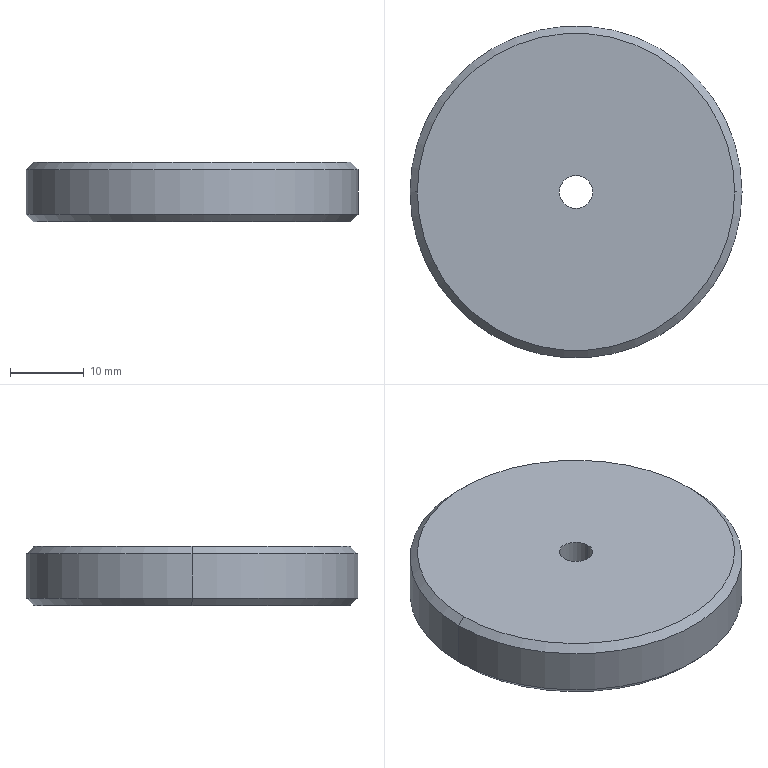Part | STEP file | SPM 1 | 1 solid | 13 faces | box 45 x 45 x 8 mm | volume 12306 mm3 | cylinder 6 | cone 4 | plane 3 | commonest cylinder face diameters 4.5 x2 8 x2 45 x2
STEP:
#1=CARTESIAN_POINT('',(0.,0.,0.));
#2=DIRECTION('',(0.,0.,1.));
#3=DIRECTION('',(1.,0.,0.));
#4=AXIS2_PLACEMENT_3D('',#1,#2,#3);
#5=CARTESIAN_POINT('',(-21.5,0.,0.));
#6=VERTEX_POINT('',#5);
#7=CARTESIAN_POINT('',(21.5,0.,0.));
#8=VERTEX_POINT('',#7);
#9=CARTESIAN_POINT('',(0.,0.,0.));
#10=DIRECTION('',(0.,0.,-1.));
#11=DIRECTION('',(1.,0.,0.));
#12=AXIS2_PLACEMENT_3D('',#9,#10,#11);
#13=CIRCLE('',#12,21.5);
#14=CARTESIAN_POINT('',(0.,0.,0.));
#15=DIRECTION('',(0.,0.,1.));
#16=DIRECTION('',(1.,0.,0.));
#17=AXIS2_PLACEMENT_3D('',#14,#15,#16);
#18=CONICAL_SURFACE('',#17,21.5,0.7854);
#19=CARTESIAN_POINT('',(6.283,0.));
#20=DIRECTION('',(-1.,0.));
#21=VECTOR('',#20,1.);
#22=LINE('',#19,#21);
#23=(GEOMETRIC_REPRESENTATION_CONTEXT(2)PARAMETRIC_REPRESENTATION_CONTEXT()REPRESENTATION_CONTEXT('',''));
#24=DEFINITIONAL_REPRESENTATION('',(#22),#23);
#25=PCURVE('',#18,#24);
#26=CARTESIAN_POINT('',(0.,0.,0.));
#27=DIRECTION('',(0.,0.,1.));
#28=DIRECTION('',(1.,0.,0.));
#29=AXIS2_PLACEMENT_3D('',#26,#27,#28);
#30=PLANE('',#29);
#31=CARTESIAN_POINT('',(21.5,0.));
#32=CARTESIAN_POINT('',(21.5,-37.239));
#33=CARTESIAN_POINT('',(-10.75,-18.62));
#34=CARTESIAN_POINT('',(-43.,0.));
#35=CARTESIAN_POINT('',(-10.75,18.62));
#36=CARTESIAN_POINT('',(21.5,37.239));
#37=CARTESIAN_POINT('',(21.5,0.));
#38=(BOUNDED_CURVE()B_SPLINE_CURVE(2,(#31,#32,#33,#34,#35,#36,#37),.UNSPECIFIED.,.T.,.F.)B_SPLINE_CURVE_WITH_KNOTS((1,2,2,2,2,1),(-2.094,0.,2.094,4.189,6.283,8.378),.UNSPECIFIED.)CURVE()GEOMETRIC_REPRESENTATION_ITEM()RATIONAL_B_SPLINE_CURVE((1.,0.5,1.,0.5,1.,0.5,1.))REPRESENTATION_ITEM(''));
#39=(GEOMETRIC_REPRESENTATION_CONTEXT(2)PARAMETRIC_REPRESENTATION_CONTEXT()REPRESENTATION_CONTEXT('',''));
#40=DEFINITIONAL_REPRESENTATION('',(#38),#39);
#41=PCURVE('',#30,#40);
#42=SURFACE_CURVE('',#13,(#25,#41),.PCURVE_S1.);
#43=EDGE_CURVE('',#6,#8,#42,.T.);
#44=ORIENTED_EDGE('',*,*,#43,.F.);
#45=CARTESIAN_POINT('',(-22.5,0.,1.));
#46=VERTEX_POINT('',#45);
#47=CARTESIAN_POINT('',(-21.5,0.,0.));
#48=DIRECTION('',(-0.7071,0.,0.7071));
#49=VECTOR('',#48,1.);
#50=LINE('',#47,#49);
#51=CARTESIAN_POINT('',(3.142,0.));
#52=DIRECTION('',(0.,1.));
#53=VECTOR('',#52,1.);
#54=LINE('',#51,#53);
#55=(GEOMETRIC_REPRESENTATION_CONTEXT(2)PARAMETRIC_REPRESENTATION_CONTEXT()REPRESENTATION_CONTEXT('',''));
#56=DEFINITIONAL_REPRESENTATION('',(#54),#55);
#57=PCURVE('',#18,#56);
#58=CARTESIAN_POINT('',(0.,0.,0.));
#59=DIRECTION('',(0.,0.,1.));
#60=DIRECTION('',(1.,0.,0.));
#61=AXIS2_PLACEMENT_3D('',#58,#59,#60);
#62=CONICAL_SURFACE('',#61,21.5,0.7854);
#63=CARTESIAN_POINT('',(3.142,0.));
#64=DIRECTION('',(0.,1.));
#65=VECTOR('',#64,1.);
#66=LINE('',#63,#65);
#67=(GEOMETRIC_REPRESENTATION_CONTEXT(2)PARAMETRIC_REPRESENTATION_CONTEXT()REPRESENTATION_CONTEXT('',''));
#68=DEFINITIONAL_REPRESENTATION('',(#66),#67);
#69=PCURVE('',#62,#68);
#70=SURFACE_CURVE('',#50,(#57,#69),.PCURVE_S1.);
#71=EDGE_CURVE('',#6,#46,#70,.T.);
#72=ORIENTED_EDGE('',*,*,#71,.T.);
#73=CARTESIAN_POINT('',(22.5,0.,1.));
#74=VERTEX_POINT('',#73);
#75=CARTESIAN_POINT('',(0.,0.,1.));
#76=DIRECTION('',(0.,0.,1.));
#77=DIRECTION('',(1.,0.,0.));
#78=AXIS2_PLACEMENT_3D('',#75,#76,#77);
#79=CIRCLE('',#78,22.5);
#80=CARTESIAN_POINT('',(0.,1.));
#81=DIRECTION('',(1.,0.));
#82=VECTOR('',#81,1.);
#83=LINE('',#80,#82);
#84=(GEOMETRIC_REPRESENTATION_CONTEXT(2)PARAMETRIC_REPRESENTATION_CONTEXT()REPRESENTATION_CONTEXT('',''));
#85=DEFINITIONAL_REPRESENTATION('',(#83),#84);
#86=PCURVE('',#18,#85);
#87=CARTESIAN_POINT('',(0.,0.,71.64));
#88=DIRECTION('',(0.,0.,-1.));
#89=DIRECTION('',(-1.,0.,0.));
#90=AXIS2_PLACEMENT_3D('',#87,#88,#89);
#91=CYLINDRICAL_SURFACE('',#90,22.5);
#92=CARTESIAN_POINT('',(3.142,70.64));
#93=DIRECTION('',(-1.,0.));
#94=VECTOR('',#93,1.);
#95=LINE('',#92,#94);
#96=(GEOMETRIC_REPRESENTATION_CONTEXT(2)PARAMETRIC_REPRESENTATION_CONTEXT()REPRESENTATION_CONTEXT('',''));
#97=DEFINITIONAL_REPRESENTATION('',(#95),#96);
#98=PCURVE('',#91,#97);
#99=SURFACE_CURVE('',#79,(#86,#98),.PCURVE_S1.);
#100=EDGE_CURVE('',#74,#46,#99,.T.);
#101=ORIENTED_EDGE('',*,*,#100,.F.);
#102=CARTESIAN_POINT('',(21.5,0.,0.));
#103=DIRECTION('',(0.7071,0.,0.7071));
#104=VECTOR('',#103,1.);
#105=LINE('',#102,#104);
#106=CARTESIAN_POINT('',(0.,0.));
#107=DIRECTION('',(0.,1.));
#108=VECTOR('',#107,1.);
#109=LINE('',#106,#108);
#110=(GEOMETRIC_REPRESENTATION_CONTEXT(2)PARAMETRIC_REPRESENTATION_CONTEXT()REPRESENTATION_CONTEXT('',''));
#111=DEFINITIONAL_REPRESENTATION('',(#109),#110);
#112=PCURVE('',#18,#111);
#113=CARTESIAN_POINT('',(6.283,0.));
#114=DIRECTION('',(0.,1.));
#115=VECTOR('',#114,1.);
#116=LINE('',#113,#115);
#117=(GEOMETRIC_REPRESENTATION_CONTEXT(2)PARAMETRIC_REPRESENTATION_CONTEXT()REPRESENTATION_CONTEXT('',''));
#118=DEFINITIONAL_REPRESENTATION('',(#116),#117);
#119=PCURVE('',#62,#118);
#120=SURFACE_CURVE('',#105,(#112,#119),.PCURVE_S1.);
#121=EDGE_CURVE('',#8,#74,#120,.T.);
#122=ORIENTED_EDGE('',*,*,#121,.F.);
#123=EDGE_LOOP('',(#44,#72,#101,#122));
#124=FACE_BOUND('',#123,.T.);
#125=ADVANCED_FACE('',(#124),#18,.T.);
#126=CARTESIAN_POINT('',(21.5,0.,8.));
#127=VERTEX_POINT('',#126);
#128=CARTESIAN_POINT('',(-21.5,0.,8.));
#129=VERTEX_POINT('',#128);
#130=CARTESIAN_POINT('',(0.,0.,8.));
#131=DIRECTION('',(0.,0.,1.));
#132=DIRECTION('',(1.,0.,0.));
#133=AXIS2_PLACEMENT_3D('',#130,#131,#132);
#134=CIRCLE('',#133,21.5);
#135=CARTESIAN_POINT('',(0.,0.,7.));
#136=DIRECTION('',(0.,0.,-1.));
#137=DIRECTION('',(-1.,0.,0.));
#138=AXIS2_PLACEMENT_3D('',#135,#136,#137);
#139=CONICAL_SURFACE('',#138,22.5,0.7854);
#140=CARTESIAN_POINT('',(3.142,-1.));
#141=DIRECTION('',(-1.,0.));
#142=VECTOR('',#141,1.);
#143=LINE('',#140,#142);
#144=(GEOMETRIC_REPRESENTATION_CONTEXT(2)PARAMETRIC_REPRESENTATION_CONTEXT()REPRESENTATION_CONTEXT('',''));
#145=DEFINITIONAL_REPRESENTATION('',(#143),#144);
#146=PCURVE('',#139,#145);
#147=CARTESIAN_POINT('',(0.,0.,8.));
#148=DIRECTION('',(0.,0.,1.));
#149=DIRECTION('',(1.,0.,0.));
#150=AXIS2_PLACEMENT_3D('',#147,#148,#149);
#151=PLANE('',#150);
#152=CARTESIAN_POINT('',(0.,0.));
#153=DIRECTION('',(1.,0.));
#154=AXIS2_PLACEMENT_2D('',#152,#153);
#155=CIRCLE('',#154,21.5);
#156=(GEOMETRIC_REPRESENTATION_CONTEXT(2)PARAMETRIC_REPRESENTATION_CONTEXT()REPRESENTATION_CONTEXT('',''));
#157=DEFINITIONAL_REPRESENTATION('',(#155),#156);
#158=PCURVE('',#151,#157);
#159=SURFACE_CURVE('',#134,(#146,#158),.PCURVE_S1.);
#160=EDGE_CURVE('',#127,#129,#159,.T.);
#161=ORIENTED_EDGE('',*,*,#160,.F.);
#162=CARTESIAN_POINT('',(22.5,0.,7.));
#163=VERTEX_POINT('',#162);
#164=CARTESIAN_POINT('',(22.5,0.,7.));
#165=DIRECTION('',(0.7071,0.,-0.7071));
#166=VECTOR('',#165,1.);
#167=LINE('',#164,#166);
#168=CARTESIAN_POINT('',(3.142,0.));
#169=DIRECTION('',(0.,1.));
#170=VECTOR('',#169,1.);
#171=LINE('',#168,#170);
#172=(GEOMETRIC_REPRESENTATION_CONTEXT(2)PARAMETRIC_REPRESENTATION_CONTEXT()REPRESENTATION_CONTEXT('',''));
#173=DEFINITIONAL_REPRESENTATION('',(#171),#172);
#174=PCURVE('',#139,#173);
#175=CARTESIAN_POINT('',(0.,0.,7.));
#176=DIRECTION('',(0.,0.,-1.));
#177=DIRECTION('',(-1.,0.,0.));
#178=AXIS2_PLACEMENT_3D('',#175,#176,#177);
#179=CONICAL_SURFACE('',#178,22.5,0.7854);
#180=CARTESIAN_POINT('',(3.142,0.));
#181=DIRECTION('',(0.,1.));
#182=VECTOR('',#181,1.);
#183=LINE('',#180,#182);
#184=(GEOMETRIC_REPRESENTATION_CONTEXT(2)PARAMETRIC_REPRESENTATION_CONTEXT()REPRESENTATION_CONTEXT('',''));
#185=DEFINITIONAL_REPRESENTATION('',(#183),#184);
#186=PCURVE('',#179,#185);
#187=SURFACE_CURVE('',#167,(#174,#186),.PCURVE_S1.);
#188=EDGE_CURVE('',#127,#163,#187,.T.);
#189=ORIENTED_EDGE('',*,*,#188,.T.);
#190=CARTESIAN_POINT('',(-22.5,0.,7.));
#191=VERTEX_POINT('',#190);
#192=CARTESIAN_POINT('',(0.,0.,7.));
#193=DIRECTION('',(0.,0.,-1.));
#194=DIRECTION('',(1.,0.,0.));
#195=AXIS2_PLACEMENT_3D('',#192,#193,#194);
#196=CIRCLE('',#195,22.5);
#197=CARTESIAN_POINT('',(-3.142,0.));
#198=DIRECTION('',(1.,0.));
#199=VECTOR('',#198,1.);
#200=LINE('',#197,#199);
#201=(GEOMETRIC_REPRESENTATION_CONTEXT(2)PARAMETRIC_REPRESENTATION_CONTEXT()REPRESENTATION_CONTEXT('',''));
#202=DEFINITIONAL_REPRESENTATION('',(#200),#201);
#203=PCURVE('',#139,#202);
#204=CARTESIAN_POINT('',(-3.142,64.64));
#205=DIRECTION('',(1.,0.));
#206=VECTOR('',#205,1.);
#207=LINE('',#204,#206);
#208=(GEOMETRIC_REPRESENTATION_CONTEXT(2)PARAMETRIC_REPRESENTATION_CONTEXT()REPRESENTATION_CONTEXT('',''));
#209=DEFINITIONAL_REPRESENTATION('',(#207),#208);
#210=PCURVE('',#91,#209);
#211=SURFACE_CURVE('',#196,(#203,#210),.PCURVE_S1.);
#212=EDGE_CURVE('',#191,#163,#211,.T.);
#213=ORIENTED_EDGE('',*,*,#212,.F.);
#214=CARTESIAN_POINT('',(-22.5,0.,7.));
#215=DIRECTION('',(-0.7071,0.,-0.7071));
#216=VECTOR('',#215,1.);
#217=LINE('',#214,#216);
#218=CARTESIAN_POINT('',(0.,0.));
#219=DIRECTION('',(0.,1.));
#220=VECTOR('',#219,1.);
#221=LINE('',#218,#220);
#222=(GEOMETRIC_REPRESENTATION_CONTEXT(2)PARAMETRIC_REPRESENTATION_CONTEXT()REPRESENTATION_CONTEXT('',''));
#223=DEFINITIONAL_REPRESENTATION('',(#221),#222);
#224=PCURVE('',#139,#223);
#225=CARTESIAN_POINT('',(6.283,0.));
#226=DIRECTION('',(0.,1.));
#227=VECTOR('',#226,1.);
#228=LINE('',#225,#227);
#229=(GEOMETRIC_REPRESENTATION_CONTEXT(2)PARAMETRIC_REPRESENTATION_CONTEXT()REPRESENTATION_CONTEXT('',''));
#230=DEFINITIONAL_REPRESENTATION('',(#228),#229);
#231=PCURVE('',#179,#230);
#232=SURFACE_CURVE('',#217,(#224,#231),.PCURVE_S1.);
#233=EDGE_CURVE('',#129,#191,#232,.T.);
#234=ORIENTED_EDGE('',*,*,#233,.F.);
#235=EDGE_LOOP('',(#161,#189,#213,#234));
#236=FACE_BOUND('',#235,.T.);
#237=ADVANCED_FACE('',(#236),#139,.T.);
#238=ORIENTED_EDGE('',*,*,#212,.T.);
#239=CARTESIAN_POINT('',(22.5,0.,71.64));
#240=DIRECTION('',(0.,0.,-1.));
#241=VECTOR('',#240,1.);
#242=LINE('',#239,#241);
#243=CARTESIAN_POINT('',(3.142,0.));
#244=DIRECTION('',(0.,1.));
#245=VECTOR('',#244,1.);
#246=LINE('',#243,#245);
#247=(GEOMETRIC_REPRESENTATION_CONTEXT(2)PARAMETRIC_REPRESENTATION_CONTEXT()REPRESENTATION_CONTEXT('',''));
#248=DEFINITIONAL_REPRESENTATION('',(#246),#247);
#249=PCURVE('',#91,#248);
#250=CARTESIAN_POINT('',(0.,0.,71.64));
#251=DIRECTION('',(0.,0.,-1.));
#252=DIRECTION('',(-1.,0.,0.));
#253=AXIS2_PLACEMENT_3D('',#250,#251,#252);
#254=CYLINDRICAL_SURFACE('',#253,22.5);
#255=CARTESIAN_POINT('',(3.142,0.));
#256=DIRECTION('',(0.,1.));
#257=VECTOR('',#256,1.);
#258=LINE('',#255,#257);
#259=(GEOMETRIC_REPRESENTATION_CONTEXT(2)PARAMETRIC_REPRESENTATION_CONTEXT()REPRESENTATION_CONTEXT('',''));
#260=DEFINITIONAL_REPRESENTATION('',(#258),#259);
#261=PCURVE('',#254,#260);
#262=SURFACE_CURVE('',#242,(#249,#261),.PCURVE_S1.);
#263=EDGE_CURVE('',#163,#74,#262,.T.);
#264=ORIENTED_EDGE('',*,*,#263,.T.);
#265=ORIENTED_EDGE('',*,*,#100,.T.);
#266=CARTESIAN_POINT('',(-22.5,0.,71.64));
#267=DIRECTION('',(0.,0.,-1.));
#268=VECTOR('',#267,1.);
#269=LINE('',#266,#268);
#270=CARTESIAN_POINT('',(0.,0.));
#271=DIRECTION('',(0.,1.));
#272=VECTOR('',#271,1.);
#273=LINE('',#270,#272);
#274=(GEOMETRIC_REPRESENTATION_CONTEXT(2)PARAMETRIC_REPRESENTATION_CONTEXT()REPRESENTATION_CONTEXT('',''));
#275=DEFINITIONAL_REPRESENTATION('',(#273),#274);
#276=PCURVE('',#91,#275);
#277=CARTESIAN_POINT('',(6.283,0.));
#278=DIRECTION('',(0.,1.));
#279=VECTOR('',#278,1.);
#280=LINE('',#277,#279);
#281=(GEOMETRIC_REPRESENTATION_CONTEXT(2)PARAMETRIC_REPRESENTATION_CONTEXT()REPRESENTATION_CONTEXT('',''));
#282=DEFINITIONAL_REPRESENTATION('',(#280),#281);
#283=PCURVE('',#254,#282);
#284=SURFACE_CURVE('',#269,(#276,#283),.PCURVE_S1.);
#285=EDGE_CURVE('',#191,#46,#284,.T.);
#286=ORIENTED_EDGE('',*,*,#285,.F.);
#287=EDGE_LOOP('',(#238,#264,#265,#286));
#288=FACE_BOUND('',#287,.T.);
#289=ADVANCED_FACE('',(#288),#91,.T.);
#290=CARTESIAN_POINT('',(-2.25,0.,8.));
#291=VERTEX_POINT('',#290);
#292=CARTESIAN_POINT('',(-2.25,0.,4.4));
#293=VERTEX_POINT('',#292);
#294=CARTESIAN_POINT('',(-2.25,0.,8.08));
#295=DIRECTION('',(0.,0.,-1.));
#296=VECTOR('',#295,1.);
#297=LINE('',#294,#296);
#298=CARTESIAN_POINT('',(0.,0.,8.08));
#299=DIRECTION('',(0.,0.,-1.));
#300=DIRECTION('',(-1.,0.,0.));
#301=AXIS2_PLACEMENT_3D('',#298,#299,#300);
#302=CYLINDRICAL_SURFACE('',#301,2.25);
#303=CARTESIAN_POINT('',(6.283,0.));
#304=DIRECTION('',(0.,1.));
#305=VECTOR('',#304,1.);
#306=LINE('',#303,#305);
#307=(GEOMETRIC_REPRESENTATION_CONTEXT(2)PARAMETRIC_REPRESENTATION_CONTEXT()REPRESENTATION_CONTEXT('',''));
#308=DEFINITIONAL_REPRESENTATION('',(#306),#307);
#309=PCURVE('',#302,#308);
#310=CARTESIAN_POINT('',(0.,0.,8.08));
#311=DIRECTION('',(0.,0.,-1.));
#312=DIRECTION('',(-1.,0.,0.));
#313=AXIS2_PLACEMENT_3D('',#310,#311,#312);
#314=CYLINDRICAL_SURFACE('',#313,2.25);
#315=CARTESIAN_POINT('',(0.,0.));
#316=DIRECTION('',(0.,1.));
#317=VECTOR('',#316,1.);
#318=LINE('',#315,#317);
#319=(GEOMETRIC_REPRESENTATION_CONTEXT(2)PARAMETRIC_REPRESENTATION_CONTEXT()REPRESENTATION_CONTEXT('',''));
#320=DEFINITIONAL_REPRESENTATION('',(#318),#319);
#321=PCURVE('',#314,#320);
#322=SURFACE_CURVE('',#297,(#309,#321),.PCURVE_S1.);
#323=EDGE_CURVE('',#291,#293,#322,.T.);
#324=ORIENTED_EDGE('',*,*,#323,.T.);
#325=CARTESIAN_POINT('',(2.25,0.,4.4));
#326=VERTEX_POINT('',#325);
#327=CARTESIAN_POINT('',(0.,0.,4.4));
#328=DIRECTION('',(0.,0.,1.));
#329=DIRECTION('',(1.,0.,0.));
#330=AXIS2_PLACEMENT_3D('',#327,#328,#329);
#331=CIRCLE('',#330,2.25);
#332=CARTESIAN_POINT('',(9.425,3.68));
#333=DIRECTION('',(-1.,0.));
#334=VECTOR('',#333,1.);
#335=LINE('',#332,#334);
#336=(GEOMETRIC_REPRESENTATION_CONTEXT(2)PARAMETRIC_REPRESENTATION_CONTEXT()REPRESENTATION_CONTEXT('',''));
#337=DEFINITIONAL_REPRESENTATION('',(#335),#336);
#338=PCURVE('',#302,#337);
#339=CARTESIAN_POINT('',(0.,0.,4.4));
#340=DIRECTION('',(0.,0.,1.));
#341=DIRECTION('',(1.,0.,0.));
#342=AXIS2_PLACEMENT_3D('',#339,#340,#341);
#343=PLANE('',#342);
#344=CARTESIAN_POINT('',(0.,0.));
#345=DIRECTION('',(1.,0.));
#346=AXIS2_PLACEMENT_2D('',#344,#345);
#347=CIRCLE('',#346,2.25);
#348=(GEOMETRIC_REPRESENTATION_CONTEXT(2)PARAMETRIC_REPRESENTATION_CONTEXT()REPRESENTATION_CONTEXT('',''));
#349=DEFINITIONAL_REPRESENTATION('',(#347),#348);
#350=PCURVE('',#343,#349);
#351=SURFACE_CURVE('',#331,(#338,#350),.PCURVE_S1.);
#352=EDGE_CURVE('',#293,#326,#351,.T.);
#353=ORIENTED_EDGE('',*,*,#352,.T.);
#354=CARTESIAN_POINT('',(2.25,0.,8.));
#355=VERTEX_POINT('',#354);
#356=CARTESIAN_POINT('',(2.25,0.,8.08));
#357=DIRECTION('',(0.,0.,-1.));
#358=VECTOR('',#357,1.);
#359=LINE('',#356,#358);
#360=CARTESIAN_POINT('',(3.142,0.));
#361=DIRECTION('',(0.,1.));
#362=VECTOR('',#361,1.);
#363=LINE('',#360,#362);
#364=(GEOMETRIC_REPRESENTATION_CONTEXT(2)PARAMETRIC_REPRESENTATION_CONTEXT()REPRESENTATION_CONTEXT('',''));
#365=DEFINITIONAL_REPRESENTATION('',(#363),#364);
#366=PCURVE('',#302,#365);
#367=CARTESIAN_POINT('',(3.142,0.));
#368=DIRECTION('',(0.,1.));
#369=VECTOR('',#368,1.);
#370=LINE('',#367,#369);
#371=(GEOMETRIC_REPRESENTATION_CONTEXT(2)PARAMETRIC_REPRESENTATION_CONTEXT()REPRESENTATION_CONTEXT('',''));
#372=DEFINITIONAL_REPRESENTATION('',(#370),#371);
#373=PCURVE('',#314,#372);
#374=SURFACE_CURVE('',#359,(#366,#373),.PCURVE_S1.);
#375=EDGE_CURVE('',#355,#326,#374,.T.);
#376=ORIENTED_EDGE('',*,*,#375,.F.);
#377=CARTESIAN_POINT('',(0.,0.,8.));
#378=DIRECTION('',(0.,0.,1.));
#379=DIRECTION('',(1.,0.,0.));
#380=AXIS2_PLACEMENT_3D('',#377,#378,#379);
#381=CIRCLE('',#380,2.25);
#382=CARTESIAN_POINT('',(9.425,0.08));
#383=DIRECTION('',(-1.,0.));
#384=VECTOR('',#383,1.);
#385=LINE('',#382,#384);
#386=(GEOMETRIC_REPRESENTATION_CONTEXT(2)PARAMETRIC_REPRESENTATION_CONTEXT()REPRESENTATION_CONTEXT('',''));
#387=DEFINITIONAL_REPRESENTATION('',(#385),#386);
#388=PCURVE('',#302,#387);
#389=CARTESIAN_POINT('',(0.,0.));
#390=DIRECTION('',(1.,0.));
#391=AXIS2_PLACEMENT_2D('',#389,#390);
#392=CIRCLE('',#391,2.25);
#393=(GEOMETRIC_REPRESENTATION_CONTEXT(2)PARAMETRIC_REPRESENTATION_CONTEXT()REPRESENTATION_CONTEXT('',''));
#394=DEFINITIONAL_REPRESENTATION('',(#392),#393);
#395=PCURVE('',#151,#394);
#396=SURFACE_CURVE('',#381,(#388,#395),.PCURVE_S1.);
#397=EDGE_CURVE('',#291,#355,#396,.T.);
#398=ORIENTED_EDGE('',*,*,#397,.F.);
#399=EDGE_LOOP('',(#324,#353,#376,#398));
#400=FACE_BOUND('',#399,.F.);
#401=ADVANCED_FACE('',(#400),#302,.F.);
#402=CARTESIAN_POINT('',(-4.,0.,4.4));
#403=VERTEX_POINT('',#402);
#404=CARTESIAN_POINT('',(-4.,0.,0.));
#405=VERTEX_POINT('',#404);
#406=CARTESIAN_POINT('',(-4.,0.,4.4));
#407=DIRECTION('',(0.,0.,-1.));
#408=VECTOR('',#407,1.);
#409=LINE('',#406,#408);
#410=CARTESIAN_POINT('',(0.,0.,4.4));
#411=DIRECTION('',(0.,0.,-1.));
#412=DIRECTION('',(-1.,0.,0.));
#413=AXIS2_PLACEMENT_3D('',#410,#411,#412);
#414=CYLINDRICAL_SURFACE('',#413,4.);
#415=CARTESIAN_POINT('',(6.283,0.));
#416=DIRECTION('',(0.,1.));
#417=VECTOR('',#416,1.);
#418=LINE('',#415,#417);
#419=(GEOMETRIC_REPRESENTATION_CONTEXT(2)PARAMETRIC_REPRESENTATION_CONTEXT()REPRESENTATION_CONTEXT('',''));
#420=DEFINITIONAL_REPRESENTATION('',(#418),#419);
#421=PCURVE('',#414,#420);
#422=CARTESIAN_POINT('',(0.,0.,4.4));
#423=DIRECTION('',(0.,0.,-1.));
#424=DIRECTION('',(-1.,0.,0.));
#425=AXIS2_PLACEMENT_3D('',#422,#423,#424);
#426=CYLINDRICAL_SURFACE('',#425,4.);
#427=CARTESIAN_POINT('',(0.,0.));
#428=DIRECTION('',(0.,1.));
#429=VECTOR('',#428,1.);
#430=LINE('',#427,#429);
#431=(GEOMETRIC_REPRESENTATION_CONTEXT(2)PARAMETRIC_REPRESENTATION_CONTEXT()REPRESENTATION_CONTEXT('',''));
#432=DEFINITIONAL_REPRESENTATION('',(#430),#431);
#433=PCURVE('',#426,#432);
#434=SURFACE_CURVE('',#409,(#421,#433),.PCURVE_S1.);
#435=EDGE_CURVE('',#403,#405,#434,.T.);
#436=ORIENTED_EDGE('',*,*,#435,.T.);
#437=CARTESIAN_POINT('',(4.,0.,0.));
#438=VERTEX_POINT('',#437);
#439=CARTESIAN_POINT('',(0.,0.,0.));
#440=DIRECTION('',(0.,0.,1.));
#441=DIRECTION('',(-1.,0.,0.));
#442=AXIS2_PLACEMENT_3D('',#439,#440,#441);
#443=CIRCLE('',#442,4.);
#444=CARTESIAN_POINT('',(6.283,4.4));
#445=DIRECTION('',(-1.,0.));
#446=VECTOR('',#445,1.);
#447=LINE('',#444,#446);
#448=(GEOMETRIC_REPRESENTATION_CONTEXT(2)PARAMETRIC_REPRESENTATION_CONTEXT()REPRESENTATION_CONTEXT('',''));
#449=DEFINITIONAL_REPRESENTATION('',(#447),#448);
#450=PCURVE('',#414,#449);
#451=CARTESIAN_POINT('',(0.,0.));
#452=DIRECTION('',(-1.,0.));
#453=AXIS2_PLACEMENT_2D('',#451,#452);
#454=CIRCLE('',#453,4.);
#455=(GEOMETRIC_REPRESENTATION_CONTEXT(2)PARAMETRIC_REPRESENTATION_CONTEXT()REPRESENTATION_CONTEXT('',''));
#456=DEFINITIONAL_REPRESENTATION('',(#454),#455);
#457=PCURVE('',#30,#456);
#458=SURFACE_CURVE('',#443,(#450,#457),.PCURVE_S1.);
#459=EDGE_CURVE('',#405,#438,#458,.T.);
#460=ORIENTED_EDGE('',*,*,#459,.T.);
#461=CARTESIAN_POINT('',(4.,0.,4.4));
#462=VERTEX_POINT('',#461);
#463=CARTESIAN_POINT('',(4.,0.,4.4));
#464=DIRECTION('',(0.,0.,-1.));
#465=VECTOR('',#464,1.);
#466=LINE('',#463,#465);
#467=CARTESIAN_POINT('',(3.142,0.));
#468=DIRECTION('',(0.,1.));
#469=VECTOR('',#468,1.);
#470=LINE('',#467,#469);
#471=(GEOMETRIC_REPRESENTATION_CONTEXT(2)PARAMETRIC_REPRESENTATION_CONTEXT()REPRESENTATION_CONTEXT('',''));
#472=DEFINITIONAL_REPRESENTATION('',(#470),#471);
#473=PCURVE('',#414,#472);
#474=CARTESIAN_POINT('',(3.142,0.));
#475=DIRECTION('',(0.,1.));
#476=VECTOR('',#475,1.);
#477=LINE('',#474,#476);
#478=(GEOMETRIC_REPRESENTATION_CONTEXT(2)PARAMETRIC_REPRESENTATION_CONTEXT()REPRESENTATION_CONTEXT('',''));
#479=DEFINITIONAL_REPRESENTATION('',(#477),#478);
#480=PCURVE('',#426,#479);
#481=SURFACE_CURVE('',#466,(#473,#480),.PCURVE_S1.);
#482=EDGE_CURVE('',#462,#438,#481,.T.);
#483=ORIENTED_EDGE('',*,*,#482,.F.);
#484=CARTESIAN_POINT('',(0.,0.,4.4));
#485=DIRECTION('',(0.,0.,-1.));
#486=DIRECTION('',(-1.,0.,0.));
#487=AXIS2_PLACEMENT_3D('',#484,#485,#486);
#488=CIRCLE('',#487,4.);
#489=CARTESIAN_POINT('',(0.,0.));
#490=DIRECTION('',(1.,0.));
#491=VECTOR('',#490,1.);
#492=LINE('',#489,#491);
#493=(GEOMETRIC_REPRESENTATION_CONTEXT(2)PARAMETRIC_REPRESENTATION_CONTEXT()REPRESENTATION_CONTEXT('',''));
#494=DEFINITIONAL_REPRESENTATION('',(#492),#493);
#495=PCURVE('',#414,#494);
#496=CARTESIAN_POINT('',(-4.,0.));
#497=CARTESIAN_POINT('',(-4.,6.928));
#498=CARTESIAN_POINT('',(2.,3.464));
#499=CARTESIAN_POINT('',(8.,0.));
#500=CARTESIAN_POINT('',(2.,-3.464));
#501=CARTESIAN_POINT('',(-4.,-6.928));
#502=CARTESIAN_POINT('',(-4.,0.));
#503=(BOUNDED_CURVE()B_SPLINE_CURVE(2,(#496,#497,#498,#499,#500,#501,#502),.UNSPECIFIED.,.T.,.F.)B_SPLINE_CURVE_WITH_KNOTS((1,2,2,2,2,1),(-2.094,0.,2.094,4.189,6.283,8.378),.UNSPECIFIED.)CURVE()GEOMETRIC_REPRESENTATION_ITEM()RATIONAL_B_SPLINE_CURVE((1.,0.5,1.,0.5,1.,0.5,1.))REPRESENTATION_ITEM(''));
#504=(GEOMETRIC_REPRESENTATION_CONTEXT(2)PARAMETRIC_REPRESENTATION_CONTEXT()REPRESENTATION_CONTEXT('',''));
#505=DEFINITIONAL_REPRESENTATION('',(#503),#504);
#506=PCURVE('',#343,#505);
#507=SURFACE_CURVE('',#488,(#495,#506),.PCURVE_S1.);
#508=EDGE_CURVE('',#462,#403,#507,.T.);
#509=ORIENTED_EDGE('',*,*,#508,.T.);
#510=EDGE_LOOP('',(#436,#460,#483,#509));
#511=FACE_BOUND('',#510,.F.);
#512=ADVANCED_FACE('',(#511),#414,.F.);
#513=CARTESIAN_POINT('',(0.,0.,8.));
#514=DIRECTION('',(0.,0.,1.));
#515=DIRECTION('',(1.,0.,0.));
#516=AXIS2_PLACEMENT_3D('',#513,#514,#515);
#517=CIRCLE('',#516,21.5);
#518=CARTESIAN_POINT('',(0.,0.));
#519=DIRECTION('',(1.,0.));
#520=AXIS2_PLACEMENT_2D('',#518,#519);
#521=CIRCLE('',#520,21.5);
#522=(GEOMETRIC_REPRESENTATION_CONTEXT(2)PARAMETRIC_REPRESENTATION_CONTEXT()REPRESENTATION_CONTEXT('',''));
#523=DEFINITIONAL_REPRESENTATION('',(#521),#522);
#524=PCURVE('',#151,#523);
#525=CARTESIAN_POINT('',(9.425,-1.));
#526=DIRECTION('',(-1.,0.));
#527=VECTOR('',#526,1.);
#528=LINE('',#525,#527);
#529=(GEOMETRIC_REPRESENTATION_CONTEXT(2)PARAMETRIC_REPRESENTATION_CONTEXT()REPRESENTATION_CONTEXT('',''));
#530=DEFINITIONAL_REPRESENTATION('',(#528),#529);
#531=PCURVE('',#179,#530);
#532=SURFACE_CURVE('',#517,(#524,#531),.PCURVE_S1.);
#533=EDGE_CURVE('',#129,#127,#532,.T.);
#534=ORIENTED_EDGE('',*,*,#533,.T.);
#535=ORIENTED_EDGE('',*,*,#160,.T.);
#536=EDGE_LOOP('',(#534,#535));
#537=FACE_BOUND('',#536,.T.);
#538=ORIENTED_EDGE('',*,*,#397,.F.);
#539=CARTESIAN_POINT('',(0.,0.,8.));
#540=DIRECTION('',(0.,0.,1.));
#541=DIRECTION('',(1.,0.,0.));
#542=AXIS2_PLACEMENT_3D('',#539,#540,#541);
#543=CIRCLE('',#542,2.25);
#544=CARTESIAN_POINT('',(0.,0.));
#545=DIRECTION('',(1.,0.));
#546=AXIS2_PLACEMENT_2D('',#544,#545);
#547=CIRCLE('',#546,2.25);
#548=(GEOMETRIC_REPRESENTATION_CONTEXT(2)PARAMETRIC_REPRESENTATION_CONTEXT()REPRESENTATION_CONTEXT('',''));
#549=DEFINITIONAL_REPRESENTATION('',(#547),#548);
#550=PCURVE('',#151,#549);
#551=CARTESIAN_POINT('',(3.142,0.08));
#552=DIRECTION('',(-1.,0.));
#553=VECTOR('',#552,1.);
#554=LINE('',#551,#553);
#555=(GEOMETRIC_REPRESENTATION_CONTEXT(2)PARAMETRIC_REPRESENTATION_CONTEXT()REPRESENTATION_CONTEXT('',''));
#556=DEFINITIONAL_REPRESENTATION('',(#554),#555);
#557=PCURVE('',#314,#556);
#558=SURFACE_CURVE('',#543,(#550,#557),.PCURVE_S1.);
#559=EDGE_CURVE('',#355,#291,#558,.T.);
#560=ORIENTED_EDGE('',*,*,#559,.F.);
#561=EDGE_LOOP('',(#538,#560));
#562=FACE_BOUND('',#561,.T.);
#563=ADVANCED_FACE('',(#537,#562),#151,.T.);
#564=CARTESIAN_POINT('',(0.,0.,0.));
#565=DIRECTION('',(0.,0.,-1.));
#566=DIRECTION('',(1.,0.,0.));
#567=AXIS2_PLACEMENT_3D('',#564,#565,#566);
#568=CIRCLE('',#567,21.5);
#569=CARTESIAN_POINT('',(21.5,0.));
#570=CARTESIAN_POINT('',(21.5,-37.239));
#571=CARTESIAN_POINT('',(-10.75,-18.62));
#572=CARTESIAN_POINT('',(-43.,0.));
#573=CARTESIAN_POINT('',(-10.75,18.62));
#574=CARTESIAN_POINT('',(21.5,37.239));
#575=CARTESIAN_POINT('',(21.5,0.));
#576=(BOUNDED_CURVE()B_SPLINE_CURVE(2,(#569,#570,#571,#572,#573,#574,#575),.UNSPECIFIED.,.T.,.F.)B_SPLINE_CURVE_WITH_KNOTS((1,2,2,2,2,1),(-2.094,0.,2.094,4.189,6.283,8.378),.UNSPECIFIED.)CURVE()GEOMETRIC_REPRESENTATION_ITEM()RATIONAL_B_SPLINE_CURVE((1.,0.5,1.,0.5,1.,0.5,1.))REPRESENTATION_ITEM(''));
#577=(GEOMETRIC_REPRESENTATION_CONTEXT(2)PARAMETRIC_REPRESENTATION_CONTEXT()REPRESENTATION_CONTEXT('',''));
#578=DEFINITIONAL_REPRESENTATION('',(#576),#577);
#579=PCURVE('',#30,#578);
#580=CARTESIAN_POINT('',(6.283,0.));
#581=DIRECTION('',(-1.,0.));
#582=VECTOR('',#581,1.);
#583=LINE('',#580,#582);
#584=(GEOMETRIC_REPRESENTATION_CONTEXT(2)PARAMETRIC_REPRESENTATION_CONTEXT()REPRESENTATION_CONTEXT('',''));
#585=DEFINITIONAL_REPRESENTATION('',(#583),#584);
#586=PCURVE('',#62,#585);
#587=SURFACE_CURVE('',#568,(#579,#586),.PCURVE_S1.);
#588=EDGE_CURVE('',#8,#6,#587,.T.);
#589=ORIENTED_EDGE('',*,*,#588,.T.);
#590=ORIENTED_EDGE('',*,*,#43,.T.);
#591=EDGE_LOOP('',(#589,#590));
#592=FACE_BOUND('',#591,.T.);
#593=ORIENTED_EDGE('',*,*,#459,.T.);
#594=CARTESIAN_POINT('',(0.,0.,0.));
#595=DIRECTION('',(0.,0.,1.));
#596=DIRECTION('',(-1.,0.,0.));
#597=AXIS2_PLACEMENT_3D('',#594,#595,#596);
#598=CIRCLE('',#597,4.);
#599=CARTESIAN_POINT('',(0.,0.));
#600=DIRECTION('',(-1.,0.));
#601=AXIS2_PLACEMENT_2D('',#599,#600);
#602=CIRCLE('',#601,4.);
#603=(GEOMETRIC_REPRESENTATION_CONTEXT(2)PARAMETRIC_REPRESENTATION_CONTEXT()REPRESENTATION_CONTEXT('',''));
#604=DEFINITIONAL_REPRESENTATION('',(#602),#603);
#605=PCURVE('',#30,#604);
#606=CARTESIAN_POINT('',(6.283,4.4));
#607=DIRECTION('',(-1.,0.));
#608=VECTOR('',#607,1.);
#609=LINE('',#606,#608);
#610=(GEOMETRIC_REPRESENTATION_CONTEXT(2)PARAMETRIC_REPRESENTATION_CONTEXT()REPRESENTATION_CONTEXT('',''));
#611=DEFINITIONAL_REPRESENTATION('',(#609),#610);
#612=PCURVE('',#426,#611);
#613=SURFACE_CURVE('',#598,(#605,#612),.PCURVE_S1.);
#614=EDGE_CURVE('',#438,#405,#613,.T.);
#615=ORIENTED_EDGE('',*,*,#614,.T.);
#616=EDGE_LOOP('',(#593,#615));
#617=FACE_BOUND('',#616,.T.);
#618=ADVANCED_FACE('',(#592,#617),#30,.F.);
#619=ORIENTED_EDGE('',*,*,#352,.T.);
#620=CARTESIAN_POINT('',(0.,0.,4.4));
#621=DIRECTION('',(0.,0.,1.));
#622=DIRECTION('',(1.,0.,0.));
#623=AXIS2_PLACEMENT_3D('',#620,#621,#622);
#624=CIRCLE('',#623,2.25);
#625=CARTESIAN_POINT('',(0.,0.));
#626=DIRECTION('',(1.,0.));
#627=AXIS2_PLACEMENT_2D('',#625,#626);
#628=CIRCLE('',#627,2.25);
#629=(GEOMETRIC_REPRESENTATION_CONTEXT(2)PARAMETRIC_REPRESENTATION_CONTEXT()REPRESENTATION_CONTEXT('',''));
#630=DEFINITIONAL_REPRESENTATION('',(#628),#629);
#631=PCURVE('',#343,#630);
#632=CARTESIAN_POINT('',(3.142,3.68));
#633=DIRECTION('',(-1.,0.));
#634=VECTOR('',#633,1.);
#635=LINE('',#632,#634);
#636=(GEOMETRIC_REPRESENTATION_CONTEXT(2)PARAMETRIC_REPRESENTATION_CONTEXT()REPRESENTATION_CONTEXT('',''));
#637=DEFINITIONAL_REPRESENTATION('',(#635),#636);
#638=PCURVE('',#314,#637);
#639=SURFACE_CURVE('',#624,(#631,#638),.PCURVE_S1.);
#640=EDGE_CURVE('',#326,#293,#639,.T.);
#641=ORIENTED_EDGE('',*,*,#640,.T.);
#642=EDGE_LOOP('',(#619,#641));
#643=FACE_BOUND('',#642,.T.);
#644=CARTESIAN_POINT('',(0.,0.,4.4));
#645=DIRECTION('',(0.,0.,-1.));
#646=DIRECTION('',(-1.,0.,0.));
#647=AXIS2_PLACEMENT_3D('',#644,#645,#646);
#648=CIRCLE('',#647,4.);
#649=CARTESIAN_POINT('',(-4.,0.));
#650=CARTESIAN_POINT('',(-4.,6.928));
#651=CARTESIAN_POINT('',(2.,3.464));
#652=CARTESIAN_POINT('',(8.,0.));
#653=CARTESIAN_POINT('',(2.,-3.464));
#654=CARTESIAN_POINT('',(-4.,-6.928));
#655=CARTESIAN_POINT('',(-4.,0.));
#656=(BOUNDED_CURVE()B_SPLINE_CURVE(2,(#649,#650,#651,#652,#653,#654,#655),.UNSPECIFIED.,.T.,.F.)B_SPLINE_CURVE_WITH_KNOTS((1,2,2,2,2,1),(-2.094,0.,2.094,4.189,6.283,8.378),.UNSPECIFIED.)CURVE()GEOMETRIC_REPRESENTATION_ITEM()RATIONAL_B_SPLINE_CURVE((1.,0.5,1.,0.5,1.,0.5,1.))REPRESENTATION_ITEM(''));
#657=(GEOMETRIC_REPRESENTATION_CONTEXT(2)PARAMETRIC_REPRESENTATION_CONTEXT()REPRESENTATION_CONTEXT('',''));
#658=DEFINITIONAL_REPRESENTATION('',(#656),#657);
#659=PCURVE('',#343,#658);
#660=CARTESIAN_POINT('',(0.,0.));
#661=DIRECTION('',(1.,0.));
#662=VECTOR('',#661,1.);
#663=LINE('',#660,#662);
#664=(GEOMETRIC_REPRESENTATION_CONTEXT(2)PARAMETRIC_REPRESENTATION_CONTEXT()REPRESENTATION_CONTEXT('',''));
#665=DEFINITIONAL_REPRESENTATION('',(#663),#664);
#666=PCURVE('',#426,#665);
#667=SURFACE_CURVE('',#648,(#659,#666),.PCURVE_S1.);
#668=EDGE_CURVE('',#403,#462,#667,.T.);
#669=ORIENTED_EDGE('',*,*,#668,.T.);
#670=ORIENTED_EDGE('',*,*,#508,.T.);
#671=EDGE_LOOP('',(#669,#670));
#672=FACE_BOUND('',#671,.T.);
#673=ADVANCED_FACE('',(#643,#672),#343,.F.);
#674=ORIENTED_EDGE('',*,*,#614,.T.);
#675=ORIENTED_EDGE('',*,*,#435,.F.);
#676=ORIENTED_EDGE('',*,*,#668,.T.);
#677=ORIENTED_EDGE('',*,*,#482,.T.);
#678=EDGE_LOOP('',(#674,#675,#676,#677));
#679=FACE_BOUND('',#678,.F.);
#680=ADVANCED_FACE('',(#679),#426,.F.);
#681=ORIENTED_EDGE('',*,*,#640,.T.);
#682=ORIENTED_EDGE('',*,*,#323,.F.);
#683=ORIENTED_EDGE('',*,*,#559,.F.);
#684=ORIENTED_EDGE('',*,*,#375,.T.);
#685=EDGE_LOOP('',(#681,#682,#683,#684));
#686=FACE_BOUND('',#685,.F.);
#687=ADVANCED_FACE('',(#686),#314,.F.);
#688=ORIENTED_EDGE('',*,*,#263,.F.);
#689=CARTESIAN_POINT('',(0.,0.,7.));
#690=DIRECTION('',(0.,0.,-1.));
#691=DIRECTION('',(1.,0.,0.));
#692=AXIS2_PLACEMENT_3D('',#689,#690,#691);
#693=CIRCLE('',#692,22.5);
#694=CARTESIAN_POINT('',(3.142,64.64));
#695=DIRECTION('',(1.,0.));
#696=VECTOR('',#695,1.);
#697=LINE('',#694,#696);
#698=(GEOMETRIC_REPRESENTATION_CONTEXT(2)PARAMETRIC_REPRESENTATION_CONTEXT()REPRESENTATION_CONTEXT('',''));
#699=DEFINITIONAL_REPRESENTATION('',(#697),#698);
#700=PCURVE('',#254,#699);
#701=CARTESIAN_POINT('',(3.142,0.));
#702=DIRECTION('',(1.,0.));
#703=VECTOR('',#702,1.);
#704=LINE('',#701,#703);
#705=(GEOMETRIC_REPRESENTATION_CONTEXT(2)PARAMETRIC_REPRESENTATION_CONTEXT()REPRESENTATION_CONTEXT('',''));
#706=DEFINITIONAL_REPRESENTATION('',(#704),#705);
#707=PCURVE('',#179,#706);
#708=SURFACE_CURVE('',#693,(#700,#707),.PCURVE_S1.);
#709=EDGE_CURVE('',#163,#191,#708,.T.);
#710=ORIENTED_EDGE('',*,*,#709,.T.);
#711=ORIENTED_EDGE('',*,*,#285,.T.);
#712=CARTESIAN_POINT('',(0.,0.,1.));
#713=DIRECTION('',(0.,0.,1.));
#714=DIRECTION('',(1.,0.,0.));
#715=AXIS2_PLACEMENT_3D('',#712,#713,#714);
#716=CIRCLE('',#715,22.5);
#717=CARTESIAN_POINT('',(9.425,70.64));
#718=DIRECTION('',(-1.,0.));
#719=VECTOR('',#718,1.);
#720=LINE('',#717,#719);
#721=(GEOMETRIC_REPRESENTATION_CONTEXT(2)PARAMETRIC_REPRESENTATION_CONTEXT()REPRESENTATION_CONTEXT('',''));
#722=DEFINITIONAL_REPRESENTATION('',(#720),#721);
#723=PCURVE('',#254,#722);
#724=CARTESIAN_POINT('',(0.,1.));
#725=DIRECTION('',(1.,0.));
#726=VECTOR('',#725,1.);
#727=LINE('',#724,#726);
#728=(GEOMETRIC_REPRESENTATION_CONTEXT(2)PARAMETRIC_REPRESENTATION_CONTEXT()REPRESENTATION_CONTEXT('',''));
#729=DEFINITIONAL_REPRESENTATION('',(#727),#728);
#730=PCURVE('',#62,#729);
#731=SURFACE_CURVE('',#716,(#723,#730),.PCURVE_S1.);
#732=EDGE_CURVE('',#46,#74,#731,.T.);
#733=ORIENTED_EDGE('',*,*,#732,.T.);
#734=EDGE_LOOP('',(#688,#710,#711,#733));
#735=FACE_BOUND('',#734,.T.);
#736=ADVANCED_FACE('',(#735),#254,.T.);
#737=ORIENTED_EDGE('',*,*,#188,.F.);
#738=ORIENTED_EDGE('',*,*,#533,.F.);
#739=ORIENTED_EDGE('',*,*,#233,.T.);
#740=ORIENTED_EDGE('',*,*,#709,.F.);
#741=EDGE_LOOP('',(#737,#738,#739,#740));
#742=FACE_BOUND('',#741,.T.);
#743=ADVANCED_FACE('',(#742),#179,.T.);
#744=ORIENTED_EDGE('',*,*,#71,.F.);
#745=ORIENTED_EDGE('',*,*,#588,.F.);
#746=ORIENTED_EDGE('',*,*,#121,.T.);
#747=ORIENTED_EDGE('',*,*,#732,.F.);
#748=EDGE_LOOP('',(#744,#745,#746,#747));
#749=FACE_BOUND('',#748,.T.);
#750=ADVANCED_FACE('',(#749),#62,.T.);
#751=CLOSED_SHELL('',(#125,#237,#289,#401,#512,#563,#618,#673,#680,#687,#736,#743,#750));
#752=MANIFOLD_SOLID_BREP('',#751);
#753=(LENGTH_UNIT()NAMED_UNIT(*)SI_UNIT(.MILLI.,.METRE.));
#754=UNCERTAINTY_MEASURE_WITH_UNIT(LENGTH_MEASURE(0.0000001),#753,'','');
#755=(NAMED_UNIT(*)PLANE_ANGLE_UNIT()SI_UNIT($,.RADIAN.));
#756=(NAMED_UNIT(*)SI_UNIT($,.STERADIAN.)SOLID_ANGLE_UNIT());
#757=(GEOMETRIC_REPRESENTATION_CONTEXT(3)GLOBAL_UNCERTAINTY_ASSIGNED_CONTEXT((#754))GLOBAL_UNIT_ASSIGNED_CONTEXT((#753,#755,#756))REPRESENTATION_CONTEXT('',''));
#758=ADVANCED_BREP_SHAPE_REPRESENTATION('',(#4,#752),#757);